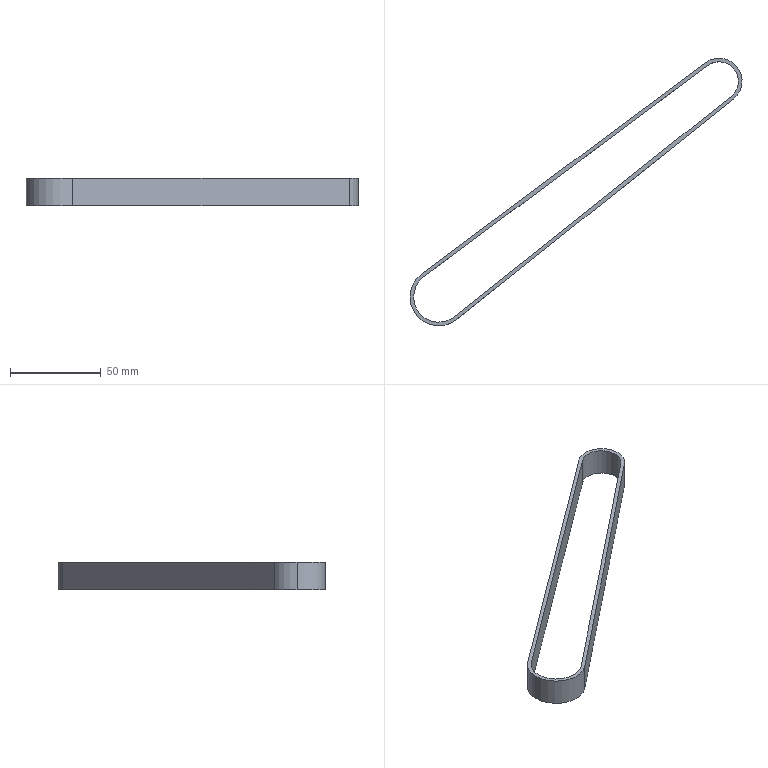Part | SolidWorks | features BaseBody 1 | 1 solid | 12 faces | box 182.982 x 147.508 x 15 mm | volume 14200 mm3 | plane 6 | cylinder 6 | commonest cylinder face diameters 27.69 x2 31.69 x2 21.32 x1 25.32 x1
STEP:
#1=CARTESIAN_POINT('',(-129.584,251.35,-7.5));
#2=VERTEX_POINT('',#1);
#3=CARTESIAN_POINT('',(-285.964,134.901,-7.5));
#4=VERTEX_POINT('',#3);
#5=CARTESIAN_POINT('',(-285.964,134.901,-7.5));
#6=DIRECTION('',(-0.8021,-0.5973,0.));
#7=VECTOR('',#6,1000.);
#8=LINE('',#5,#7);
#9=EDGE_CURVE('',#2,#4,#8,.T.);
#10=ORIENTED_EDGE('',*,*,#9,.F.);
#11=CARTESIAN_POINT('',(-129.584,251.35,7.5));
#12=VERTEX_POINT('',#11);
#13=CARTESIAN_POINT('',(-129.584,251.35,7.5));
#14=DIRECTION('',(0.,0.,-1.));
#15=VECTOR('',#14,1000.);
#16=LINE('',#13,#15);
#17=EDGE_CURVE('',#12,#2,#16,.T.);
#18=ORIENTED_EDGE('',*,*,#17,.F.);
#19=CARTESIAN_POINT('',(-285.964,134.901,7.5));
#20=VERTEX_POINT('',#19);
#21=CARTESIAN_POINT('',(-285.964,134.901,7.5));
#22=DIRECTION('',(-0.8021,-0.5973,0.));
#23=VECTOR('',#22,1000.);
#24=LINE('',#21,#23);
#25=EDGE_CURVE('',#12,#20,#24,.T.);
#26=ORIENTED_EDGE('',*,*,#25,.T.);
#27=CARTESIAN_POINT('',(-285.964,134.901,7.5));
#28=DIRECTION('',(0.,0.,-1.));
#29=VECTOR('',#28,1000.);
#30=LINE('',#27,#29);
#31=EDGE_CURVE('',#20,#4,#30,.T.);
#32=ORIENTED_EDGE('',*,*,#31,.T.);
#33=EDGE_LOOP('',(#10,#18,#26,#32));
#34=FACE_OUTER_BOUND('',#33,.T.);
#35=CARTESIAN_POINT('',(-285.964,134.901,7.5));
#36=DIRECTION('',(0.5973,-0.8021,0.));
#37=DIRECTION('',(0.,0.,-1.));
#38=AXIS2_PLACEMENT_3D('',#35,#36,#37);
#39=PLANE('',#38);
#40=ADVANCED_FACE('',(#34),#39,.T.);
#41=CARTESIAN_POINT('',(-116.575,234.463,-7.5));
#42=VERTEX_POINT('',#41);
#43=CARTESIAN_POINT('',(-123.218,242.8,-7.5));
#44=DIRECTION('',(0.,0.,1.));
#45=DIRECTION('',(-1.,0.,0.));
#46=AXIS2_PLACEMENT_3D('',#43,#44,#45);
#47=CIRCLE('',#46,10.66);
#48=EDGE_CURVE('',#42,#2,#47,.T.);
#49=ORIENTED_EDGE('',*,*,#48,.F.);
#50=CARTESIAN_POINT('',(-116.575,234.463,7.5));
#51=VERTEX_POINT('',#50);
#52=CARTESIAN_POINT('',(-116.575,234.463,7.5));
#53=DIRECTION('',(0.,0.,-1.));
#54=VECTOR('',#53,1000.);
#55=LINE('',#52,#54);
#56=EDGE_CURVE('',#51,#42,#55,.T.);
#57=ORIENTED_EDGE('',*,*,#56,.F.);
#58=CARTESIAN_POINT('',(-123.218,242.8,7.5));
#59=DIRECTION('',(0.,0.,1.));
#60=DIRECTION('',(-1.,0.,0.));
#61=AXIS2_PLACEMENT_3D('',#58,#59,#60);
#62=CIRCLE('',#61,10.66);
#63=EDGE_CURVE('',#51,#12,#62,.T.);
#64=ORIENTED_EDGE('',*,*,#63,.T.);
#65=ORIENTED_EDGE('',*,*,#17,.T.);
#66=EDGE_LOOP('',(#49,#57,#64,#65));
#67=FACE_OUTER_BOUND('',#66,.T.);
#68=CARTESIAN_POINT('',(-123.218,242.8,7.5));
#69=DIRECTION('',(0.,0.,-1.));
#70=DIRECTION('',(-1.,0.,0.));
#71=AXIS2_PLACEMENT_3D('',#68,#69,#70);
#72=CYLINDRICAL_SURFACE('',#71,10.66);
#73=ADVANCED_FACE('',(#67),#72,.F.);
#74=CARTESIAN_POINT('',(-269.068,112.968,-7.5));
#75=VERTEX_POINT('',#74);
#76=CARTESIAN_POINT('',(-116.575,234.463,-7.5));
#77=DIRECTION('',(0.7821,0.6231,0.));
#78=VECTOR('',#77,1000.);
#79=LINE('',#76,#78);
#80=EDGE_CURVE('',#75,#42,#79,.T.);
#81=ORIENTED_EDGE('',*,*,#80,.F.);
#82=CARTESIAN_POINT('',(-269.068,112.968,7.5));
#83=VERTEX_POINT('',#82);
#84=CARTESIAN_POINT('',(-269.068,112.968,7.5));
#85=DIRECTION('',(0.,0.,-1.));
#86=VECTOR('',#85,1000.);
#87=LINE('',#84,#86);
#88=EDGE_CURVE('',#83,#75,#87,.T.);
#89=ORIENTED_EDGE('',*,*,#88,.F.);
#90=CARTESIAN_POINT('',(-116.575,234.463,7.5));
#91=DIRECTION('',(0.7821,0.6231,0.));
#92=VECTOR('',#91,1000.);
#93=LINE('',#90,#92);
#94=EDGE_CURVE('',#83,#51,#93,.T.);
#95=ORIENTED_EDGE('',*,*,#94,.T.);
#96=ORIENTED_EDGE('',*,*,#56,.T.);
#97=EDGE_LOOP('',(#81,#89,#95,#96));
#98=FACE_OUTER_BOUND('',#97,.T.);
#99=CARTESIAN_POINT('',(-116.575,234.463,7.5));
#100=DIRECTION('',(-0.6231,0.7821,0.));
#101=DIRECTION('',(0.,0.,1.));
#102=AXIS2_PLACEMENT_3D('',#99,#100,#101);
#103=PLANE('',#102);
#104=ADVANCED_FACE('',(#98),#103,.T.);
#105=CARTESIAN_POINT('',(-291.54,123.797,7.5));
#106=VERTEX_POINT('',#105);
#107=CARTESIAN_POINT('',(-291.54,123.797,-7.5));
#108=VERTEX_POINT('',#107);
#109=CARTESIAN_POINT('',(-291.54,123.797,7.5));
#110=DIRECTION('',(0.,0.,-1.));
#111=VECTOR('',#110,1000.);
#112=LINE('',#109,#111);
#113=EDGE_CURVE('',#106,#108,#112,.T.);
#114=ORIENTED_EDGE('',*,*,#113,.F.);
#115=CARTESIAN_POINT('',(-277.695,123.797,7.5));
#116=DIRECTION('',(0.,0.,1.));
#117=DIRECTION('',(-1.,0.,0.));
#118=AXIS2_PLACEMENT_3D('',#115,#116,#117);
#119=CIRCLE('',#118,13.845);
#120=EDGE_CURVE('',#106,#83,#119,.T.);
#121=ORIENTED_EDGE('',*,*,#120,.T.);
#122=ORIENTED_EDGE('',*,*,#88,.T.);
#123=CARTESIAN_POINT('',(-277.695,123.797,-7.5));
#124=DIRECTION('',(0.,0.,1.));
#125=DIRECTION('',(-1.,0.,0.));
#126=AXIS2_PLACEMENT_3D('',#123,#124,#125);
#127=CIRCLE('',#126,13.845);
#128=EDGE_CURVE('',#108,#75,#127,.T.);
#129=ORIENTED_EDGE('',*,*,#128,.F.);
#130=EDGE_LOOP('',(#114,#121,#122,#129));
#131=FACE_OUTER_BOUND('',#130,.T.);
#132=CARTESIAN_POINT('',(-277.695,123.797,7.5));
#133=DIRECTION('',(0.,0.,-1.));
#134=DIRECTION('',(-1.,0.,0.));
#135=AXIS2_PLACEMENT_3D('',#132,#133,#134);
#136=CYLINDRICAL_SURFACE('',#135,13.845);
#137=ADVANCED_FACE('',(#131),#136,.F.);
#138=CARTESIAN_POINT('',(-130.779,252.954,-7.5));
#139=VERTEX_POINT('',#138);
#140=CARTESIAN_POINT('',(-287.158,136.505,-7.5));
#141=VERTEX_POINT('',#140);
#142=CARTESIAN_POINT('',(-287.158,136.505,-7.5));
#143=DIRECTION('',(-0.8021,-0.5973,0.));
#144=VECTOR('',#143,1000.);
#145=LINE('',#142,#144);
#146=EDGE_CURVE('',#139,#141,#145,.T.);
#147=ORIENTED_EDGE('',*,*,#146,.T.);
#148=CARTESIAN_POINT('',(-287.158,136.505,7.5));
#149=VERTEX_POINT('',#148);
#150=CARTESIAN_POINT('',(-287.158,136.505,7.5));
#151=DIRECTION('',(0.,0.,-1.));
#152=VECTOR('',#151,1000.);
#153=LINE('',#150,#152);
#154=EDGE_CURVE('',#149,#141,#153,.T.);
#155=ORIENTED_EDGE('',*,*,#154,.F.);
#156=CARTESIAN_POINT('',(-130.779,252.954,7.5));
#157=VERTEX_POINT('',#156);
#158=CARTESIAN_POINT('',(-287.158,136.505,7.5));
#159=DIRECTION('',(-0.8021,-0.5973,0.));
#160=VECTOR('',#159,1000.);
#161=LINE('',#158,#160);
#162=EDGE_CURVE('',#157,#149,#161,.T.);
#163=ORIENTED_EDGE('',*,*,#162,.F.);
#164=CARTESIAN_POINT('',(-130.779,252.954,7.5));
#165=DIRECTION('',(0.,0.,-1.));
#166=VECTOR('',#165,1000.);
#167=LINE('',#164,#166);
#168=EDGE_CURVE('',#157,#139,#167,.T.);
#169=ORIENTED_EDGE('',*,*,#168,.T.);
#170=EDGE_LOOP('',(#147,#155,#163,#169));
#171=FACE_OUTER_BOUND('',#170,.T.);
#172=CARTESIAN_POINT('',(-287.158,136.505,7.5));
#173=DIRECTION('',(0.5973,-0.8021,0.));
#174=DIRECTION('',(0.,0.,-1.));
#175=AXIS2_PLACEMENT_3D('',#172,#173,#174);
#176=PLANE('',#175);
#177=ADVANCED_FACE('',(#171),#176,.F.);
#178=CARTESIAN_POINT('',(-115.329,232.898,-7.5));
#179=VERTEX_POINT('',#178);
#180=CARTESIAN_POINT('',(-123.218,242.8,-7.5));
#181=DIRECTION('',(0.,0.,1.));
#182=DIRECTION('',(-1.,0.,0.));
#183=AXIS2_PLACEMENT_3D('',#180,#181,#182);
#184=CIRCLE('',#183,12.66);
#185=EDGE_CURVE('',#179,#139,#184,.T.);
#186=ORIENTED_EDGE('',*,*,#185,.T.);
#187=ORIENTED_EDGE('',*,*,#168,.F.);
#188=CARTESIAN_POINT('',(-115.329,232.898,7.5));
#189=VERTEX_POINT('',#188);
#190=CARTESIAN_POINT('',(-123.218,242.8,7.5));
#191=DIRECTION('',(0.,0.,1.));
#192=DIRECTION('',(-1.,0.,0.));
#193=AXIS2_PLACEMENT_3D('',#190,#191,#192);
#194=CIRCLE('',#193,12.66);
#195=EDGE_CURVE('',#189,#157,#194,.T.);
#196=ORIENTED_EDGE('',*,*,#195,.F.);
#197=CARTESIAN_POINT('',(-115.329,232.898,7.5));
#198=DIRECTION('',(0.,0.,-1.));
#199=VECTOR('',#198,1000.);
#200=LINE('',#197,#199);
#201=EDGE_CURVE('',#189,#179,#200,.T.);
#202=ORIENTED_EDGE('',*,*,#201,.T.);
#203=EDGE_LOOP('',(#186,#187,#196,#202));
#204=FACE_OUTER_BOUND('',#203,.T.);
#205=CARTESIAN_POINT('',(-123.218,242.8,7.5));
#206=DIRECTION('',(0.,0.,-1.));
#207=DIRECTION('',(-1.,0.,0.));
#208=AXIS2_PLACEMENT_3D('',#205,#206,#207);
#209=CYLINDRICAL_SURFACE('',#208,12.66);
#210=ADVANCED_FACE('',(#204),#209,.T.);
#211=CARTESIAN_POINT('',(-267.821,111.404,-7.5));
#212=VERTEX_POINT('',#211);
#213=CARTESIAN_POINT('',(-267.821,111.404,-7.5));
#214=DIRECTION('',(0.7821,0.6231,0.));
#215=VECTOR('',#214,1000.);
#216=LINE('',#213,#215);
#217=EDGE_CURVE('',#212,#179,#216,.T.);
#218=ORIENTED_EDGE('',*,*,#217,.T.);
#219=ORIENTED_EDGE('',*,*,#201,.F.);
#220=CARTESIAN_POINT('',(-267.821,111.404,7.5));
#221=VERTEX_POINT('',#220);
#222=CARTESIAN_POINT('',(-267.821,111.404,7.5));
#223=DIRECTION('',(0.7821,0.6231,0.));
#224=VECTOR('',#223,1000.);
#225=LINE('',#222,#224);
#226=EDGE_CURVE('',#221,#189,#225,.T.);
#227=ORIENTED_EDGE('',*,*,#226,.F.);
#228=CARTESIAN_POINT('',(-267.821,111.404,7.5));
#229=DIRECTION('',(0.,0.,-1.));
#230=VECTOR('',#229,1000.);
#231=LINE('',#228,#230);
#232=EDGE_CURVE('',#221,#212,#231,.T.);
#233=ORIENTED_EDGE('',*,*,#232,.T.);
#234=EDGE_LOOP('',(#218,#219,#227,#233));
#235=FACE_OUTER_BOUND('',#234,.T.);
#236=CARTESIAN_POINT('',(-267.821,111.404,7.5));
#237=DIRECTION('',(-0.6231,0.7821,0.));
#238=DIRECTION('',(0.,0.,1.));
#239=AXIS2_PLACEMENT_3D('',#236,#237,#238);
#240=PLANE('',#239);
#241=ADVANCED_FACE('',(#235),#240,.F.);
#242=CARTESIAN_POINT('',(-293.54,123.797,7.5));
#243=VERTEX_POINT('',#242);
#244=CARTESIAN_POINT('',(-293.54,123.797,-7.5));
#245=VERTEX_POINT('',#244);
#246=CARTESIAN_POINT('',(-293.54,123.797,7.5));
#247=DIRECTION('',(0.,0.,-1.));
#248=VECTOR('',#247,1000.);
#249=LINE('',#246,#248);
#250=EDGE_CURVE('',#243,#245,#249,.T.);
#251=ORIENTED_EDGE('',*,*,#250,.F.);
#252=CARTESIAN_POINT('',(-277.695,123.797,7.5));
#253=DIRECTION('',(0.,0.,1.));
#254=DIRECTION('',(-1.,0.,0.));
#255=AXIS2_PLACEMENT_3D('',#252,#253,#254);
#256=CIRCLE('',#255,15.845);
#257=EDGE_CURVE('',#149,#243,#256,.T.);
#258=ORIENTED_EDGE('',*,*,#257,.F.);
#259=ORIENTED_EDGE('',*,*,#154,.T.);
#260=CARTESIAN_POINT('',(-277.695,123.797,-7.5));
#261=DIRECTION('',(0.,0.,1.));
#262=DIRECTION('',(-1.,0.,0.));
#263=AXIS2_PLACEMENT_3D('',#260,#261,#262);
#264=CIRCLE('',#263,15.845);
#265=EDGE_CURVE('',#141,#245,#264,.T.);
#266=ORIENTED_EDGE('',*,*,#265,.T.);
#267=EDGE_LOOP('',(#251,#258,#259,#266));
#268=FACE_OUTER_BOUND('',#267,.T.);
#269=CARTESIAN_POINT('',(-277.695,123.797,7.5));
#270=DIRECTION('',(0.,0.,-1.));
#271=DIRECTION('',(-1.,0.,0.));
#272=AXIS2_PLACEMENT_3D('',#269,#270,#271);
#273=CYLINDRICAL_SURFACE('',#272,15.845);
#274=ADVANCED_FACE('',(#268),#273,.T.);
#275=ORIENTED_EDGE('',*,*,#9,.T.);
#276=CARTESIAN_POINT('',(-277.695,123.797,-7.5));
#277=DIRECTION('',(0.,0.,1.));
#278=DIRECTION('',(-1.,0.,0.));
#279=AXIS2_PLACEMENT_3D('',#276,#277,#278);
#280=CIRCLE('',#279,13.845);
#281=EDGE_CURVE('',#4,#108,#280,.T.);
#282=ORIENTED_EDGE('',*,*,#281,.T.);
#283=ORIENTED_EDGE('',*,*,#128,.T.);
#284=ORIENTED_EDGE('',*,*,#80,.T.);
#285=ORIENTED_EDGE('',*,*,#48,.T.);
#286=EDGE_LOOP('',(#275,#282,#283,#284,#285));
#287=FACE_BOUND('',#286,.T.);
#288=ORIENTED_EDGE('',*,*,#265,.F.);
#289=ORIENTED_EDGE('',*,*,#146,.F.);
#290=ORIENTED_EDGE('',*,*,#185,.F.);
#291=ORIENTED_EDGE('',*,*,#217,.F.);
#292=CARTESIAN_POINT('',(-277.695,123.797,-7.5));
#293=DIRECTION('',(0.,0.,1.));
#294=DIRECTION('',(-1.,0.,0.));
#295=AXIS2_PLACEMENT_3D('',#292,#293,#294);
#296=CIRCLE('',#295,15.845);
#297=EDGE_CURVE('',#245,#212,#296,.T.);
#298=ORIENTED_EDGE('',*,*,#297,.F.);
#299=EDGE_LOOP('',(#288,#289,#290,#291,#298));
#300=FACE_OUTER_BOUND('',#299,.T.);
#301=CARTESIAN_POINT('',(-277.695,123.797,-7.5));
#302=DIRECTION('',(0.,0.,-1.));
#303=DIRECTION('',(0.,-1.,0.));
#304=AXIS2_PLACEMENT_3D('',#301,#302,#303);
#305=PLANE('',#304);
#306=ADVANCED_FACE('',(#287,#300),#305,.T.);
#307=CARTESIAN_POINT('',(-277.695,123.797,7.5));
#308=DIRECTION('',(0.,0.,1.));
#309=DIRECTION('',(-1.,0.,0.));
#310=AXIS2_PLACEMENT_3D('',#307,#308,#309);
#311=CIRCLE('',#310,13.845);
#312=EDGE_CURVE('',#20,#106,#311,.T.);
#313=ORIENTED_EDGE('',*,*,#312,.F.);
#314=ORIENTED_EDGE('',*,*,#25,.F.);
#315=ORIENTED_EDGE('',*,*,#63,.F.);
#316=ORIENTED_EDGE('',*,*,#94,.F.);
#317=ORIENTED_EDGE('',*,*,#120,.F.);
#318=EDGE_LOOP('',(#313,#314,#315,#316,#317));
#319=FACE_BOUND('',#318,.T.);
#320=ORIENTED_EDGE('',*,*,#257,.T.);
#321=CARTESIAN_POINT('',(-277.695,123.797,7.5));
#322=DIRECTION('',(0.,0.,1.));
#323=DIRECTION('',(-1.,0.,0.));
#324=AXIS2_PLACEMENT_3D('',#321,#322,#323);
#325=CIRCLE('',#324,15.845);
#326=EDGE_CURVE('',#243,#221,#325,.T.);
#327=ORIENTED_EDGE('',*,*,#326,.T.);
#328=ORIENTED_EDGE('',*,*,#226,.T.);
#329=ORIENTED_EDGE('',*,*,#195,.T.);
#330=ORIENTED_EDGE('',*,*,#162,.T.);
#331=EDGE_LOOP('',(#320,#327,#328,#329,#330));
#332=FACE_OUTER_BOUND('',#331,.T.);
#333=CARTESIAN_POINT('',(-277.695,123.797,7.5));
#334=DIRECTION('',(0.,0.,-1.));
#335=DIRECTION('',(0.,-1.,0.));
#336=AXIS2_PLACEMENT_3D('',#333,#334,#335);
#337=PLANE('',#336);
#338=ADVANCED_FACE('',(#319,#332),#337,.F.);
#339=ORIENTED_EDGE('',*,*,#326,.F.);
#340=ORIENTED_EDGE('',*,*,#250,.T.);
#341=ORIENTED_EDGE('',*,*,#297,.T.);
#342=ORIENTED_EDGE('',*,*,#232,.F.);
#343=EDGE_LOOP('',(#339,#340,#341,#342));
#344=FACE_OUTER_BOUND('',#343,.T.);
#345=CARTESIAN_POINT('',(-277.695,123.797,7.5));
#346=DIRECTION('',(0.,0.,-1.));
#347=DIRECTION('',(-1.,0.,0.));
#348=AXIS2_PLACEMENT_3D('',#345,#346,#347);
#349=CYLINDRICAL_SURFACE('',#348,15.845);
#350=ADVANCED_FACE('',(#344),#349,.T.);
#351=ORIENTED_EDGE('',*,*,#312,.T.);
#352=ORIENTED_EDGE('',*,*,#113,.T.);
#353=ORIENTED_EDGE('',*,*,#281,.F.);
#354=ORIENTED_EDGE('',*,*,#31,.F.);
#355=EDGE_LOOP('',(#351,#352,#353,#354));
#356=FACE_OUTER_BOUND('',#355,.T.);
#357=CARTESIAN_POINT('',(-277.695,123.797,7.5));
#358=DIRECTION('',(0.,0.,-1.));
#359=DIRECTION('',(-1.,0.,0.));
#360=AXIS2_PLACEMENT_3D('',#357,#358,#359);
#361=CYLINDRICAL_SURFACE('',#360,13.845);
#362=ADVANCED_FACE('',(#356),#361,.F.);
#363=CLOSED_SHELL('',(#40,#73,#104,#137,#177,#210,#241,#274,#306,#338,#350,#362));
#364=MANIFOLD_SOLID_BREP('',#363);
#365=CARTESIAN_POINT('',(0.,0.,0.));
#366=DIRECTION('',(0.,0.,1.));
#367=DIRECTION('',(1.,0.,0.));
#368=AXIS2_PLACEMENT_3D('',#365,#366,#367);
#369=(LENGTH_UNIT()NAMED_UNIT(*)SI_UNIT(.MILLI.,.METRE.));
#370=UNCERTAINTY_MEASURE_WITH_UNIT(LENGTH_MEASURE(0.00001),#369,'','');
#371=(NAMED_UNIT(*)PLANE_ANGLE_UNIT()SI_UNIT($,.RADIAN.));
#372=(NAMED_UNIT(*)SI_UNIT($,.STERADIAN.)SOLID_ANGLE_UNIT());
#373=(GEOMETRIC_REPRESENTATION_CONTEXT(3)GLOBAL_UNCERTAINTY_ASSIGNED_CONTEXT((#370))GLOBAL_UNIT_ASSIGNED_CONTEXT((#369,#371,#372))REPRESENTATION_CONTEXT('',''));
#374=ADVANCED_BREP_SHAPE_REPRESENTATION('',(#364,#368),#373);